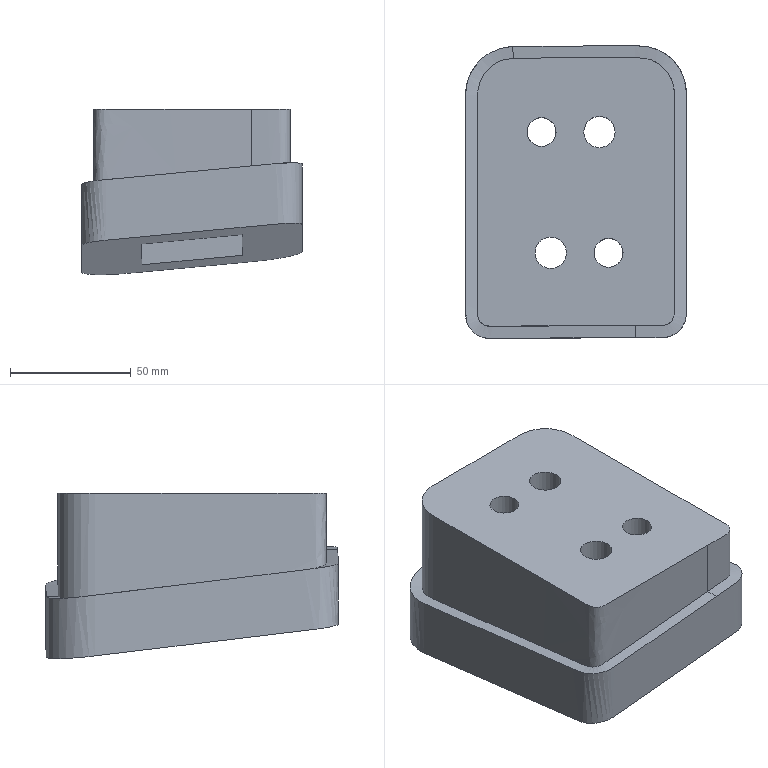Part | NX | features solid 2 | 1 solid | 22 faces | box 91.722 x 121.411 x 68.658 mm | volume 516223 mm3 | spline 13 | cylinder 6 | plane 3 | commonest cylinder face diameters 12 x2 13 x2 20 x2